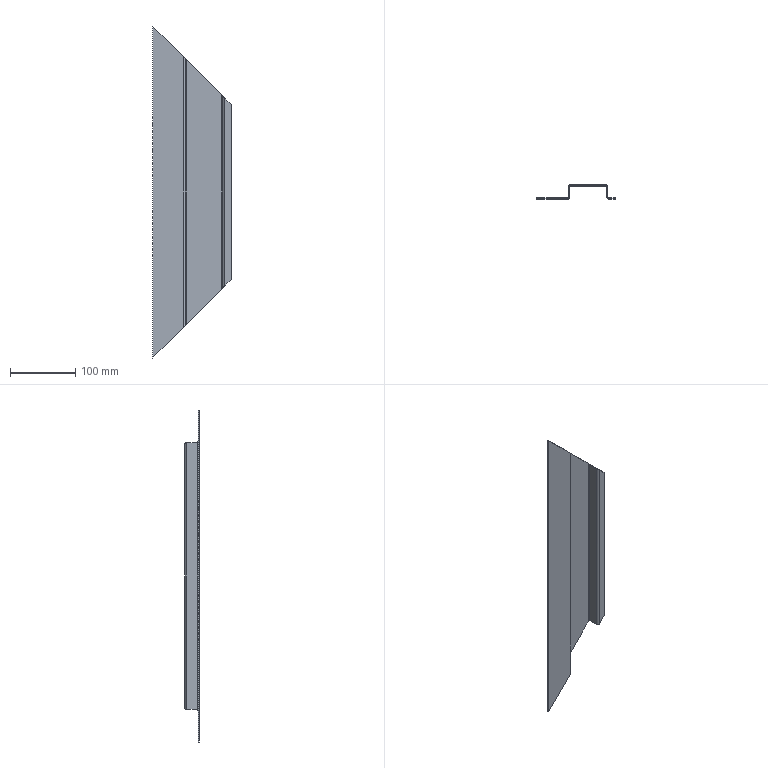Part | STEP file | 750038523 | 1 solid | 38 faces | box 120 x 21.5 x 508 mm | volume 88776 mm3 | plane 22 | cylinder 8 | spline 8 | commonest cylinder face diameters 3 x4 6 x4
STEP:
#1=CARTESIAN_POINT('',(-120.,-1.5,254.));
#2=VERTEX_POINT('',#1);
#3=CARTESIAN_POINT('',(-120.,-1.5,-254.));
#4=VERTEX_POINT('',#3);
#5=CARTESIAN_POINT('',(-120.,-1.5,254.));
#6=DIRECTION('',(0.,0.,-1.));
#7=VECTOR('',#6,1000.);
#8=LINE('',#5,#7);
#9=EDGE_CURVE('',#2,#4,#8,.T.);
#10=ORIENTED_EDGE('',*,*,#9,.T.);
#11=CARTESIAN_POINT('',(-73.,-1.5,-207.));
#12=VERTEX_POINT('',#11);
#13=CARTESIAN_POINT('',(-120.,-1.5,-254.));
#14=DIRECTION('',(0.7071,0.,0.7071));
#15=VECTOR('',#14,1000.);
#16=LINE('',#13,#15);
#17=EDGE_CURVE('',#4,#12,#16,.T.);
#18=ORIENTED_EDGE('',*,*,#17,.T.);
#19=CARTESIAN_POINT('',(-73.,-1.5,207.));
#20=VERTEX_POINT('',#19);
#21=CARTESIAN_POINT('',(-73.,-1.5,254.));
#22=DIRECTION('',(0.,0.,1.));
#23=VECTOR('',#22,1000.);
#24=LINE('',#21,#23);
#25=EDGE_CURVE('',#12,#20,#24,.T.);
#26=ORIENTED_EDGE('',*,*,#25,.T.);
#27=CARTESIAN_POINT('',(-73.,-1.5,207.));
#28=DIRECTION('',(-0.7071,0.,0.7071));
#29=VECTOR('',#28,1000.);
#30=LINE('',#27,#29);
#31=EDGE_CURVE('',#20,#2,#30,.T.);
#32=ORIENTED_EDGE('',*,*,#31,.T.);
#33=EDGE_LOOP('',(#10,#18,#26,#32));
#34=FACE_OUTER_BOUND('',#33,.T.);
#35=CARTESIAN_POINT('',(-71.5,-1.5,254.));
#36=DIRECTION('',(0.,-1.,0.));
#37=DIRECTION('',(1.,0.,0.));
#38=AXIS2_PLACEMENT_3D('',#35,#36,#37);
#39=PLANE('',#38);
#40=ADVANCED_FACE('',(#34),#39,.T.);
#41=CARTESIAN_POINT('',(-73.,0.,-207.));
#42=VERTEX_POINT('',#41);
#43=CARTESIAN_POINT('',(-73.,-0.75,-207.));
#44=DIRECTION('',(0.,-1.,0.));
#45=VECTOR('',#44,1000.);
#46=LINE('',#43,#45);
#47=EDGE_CURVE('',#42,#12,#46,.T.);
#48=ORIENTED_EDGE('',*,*,#47,.T.);
#49=ORIENTED_EDGE('',*,*,#17,.F.);
#50=CARTESIAN_POINT('',(-120.,0.,-254.));
#51=VERTEX_POINT('',#50);
#52=CARTESIAN_POINT('',(-120.,0.,-254.));
#53=DIRECTION('',(0.,1.,0.));
#54=VECTOR('',#53,1000.);
#55=LINE('',#52,#54);
#56=EDGE_CURVE('',#4,#51,#55,.T.);
#57=ORIENTED_EDGE('',*,*,#56,.T.);
#58=CARTESIAN_POINT('',(158.25,0.,24.25));
#59=DIRECTION('',(0.7071,0.,0.7071));
#60=VECTOR('',#59,1000.);
#61=LINE('',#58,#60);
#62=EDGE_CURVE('',#51,#42,#61,.T.);
#63=ORIENTED_EDGE('',*,*,#62,.T.);
#64=EDGE_LOOP('',(#48,#49,#57,#63));
#65=FACE_OUTER_BOUND('',#64,.T.);
#66=CARTESIAN_POINT('',(158.25,0.,24.25));
#67=DIRECTION('',(0.7071,0.,-0.7071));
#68=DIRECTION('',(-0.7071,0.,-0.7071));
#69=AXIS2_PLACEMENT_3D('',#66,#67,#68);
#70=PLANE('',#69);
#71=ADVANCED_FACE('',(#65),#70,.T.);
#72=ORIENTED_EDGE('',*,*,#56,.F.);
#73=ORIENTED_EDGE('',*,*,#9,.F.);
#74=CARTESIAN_POINT('',(-120.,0.,254.));
#75=VERTEX_POINT('',#74);
#76=CARTESIAN_POINT('',(-120.,0.,254.));
#77=DIRECTION('',(0.,1.,0.));
#78=VECTOR('',#77,1000.);
#79=LINE('',#76,#78);
#80=EDGE_CURVE('',#2,#75,#79,.T.);
#81=ORIENTED_EDGE('',*,*,#80,.T.);
#82=CARTESIAN_POINT('',(-120.,0.,254.));
#83=DIRECTION('',(0.,0.,-1.));
#84=VECTOR('',#83,1000.);
#85=LINE('',#82,#84);
#86=EDGE_CURVE('',#75,#51,#85,.T.);
#87=ORIENTED_EDGE('',*,*,#86,.T.);
#88=EDGE_LOOP('',(#72,#73,#81,#87));
#89=FACE_OUTER_BOUND('',#88,.T.);
#90=CARTESIAN_POINT('',(-120.,0.,254.));
#91=DIRECTION('',(-1.,0.,0.));
#92=DIRECTION('',(0.,-1.,0.));
#93=AXIS2_PLACEMENT_3D('',#90,#91,#92);
#94=PLANE('',#93);
#95=ADVANCED_FACE('',(#89),#94,.T.);
#96=ORIENTED_EDGE('',*,*,#80,.F.);
#97=ORIENTED_EDGE('',*,*,#31,.F.);
#98=CARTESIAN_POINT('',(-73.,0.,207.));
#99=VERTEX_POINT('',#98);
#100=CARTESIAN_POINT('',(-73.,-0.75,207.));
#101=DIRECTION('',(0.,1.,0.));
#102=VECTOR('',#101,1000.);
#103=LINE('',#100,#102);
#104=EDGE_CURVE('',#20,#99,#103,.T.);
#105=ORIENTED_EDGE('',*,*,#104,.T.);
#106=CARTESIAN_POINT('',(-95.75,0.,229.75));
#107=DIRECTION('',(-0.7071,0.,0.7071));
#108=VECTOR('',#107,1000.);
#109=LINE('',#106,#108);
#110=EDGE_CURVE('',#99,#75,#109,.T.);
#111=ORIENTED_EDGE('',*,*,#110,.T.);
#112=EDGE_LOOP('',(#96,#97,#105,#111));
#113=FACE_OUTER_BOUND('',#112,.T.);
#114=CARTESIAN_POINT('',(-95.75,0.,229.75));
#115=DIRECTION('',(0.7071,0.,0.7071));
#116=DIRECTION('',(0.7071,0.,-0.7071));
#117=AXIS2_PLACEMENT_3D('',#114,#115,#116);
#118=PLANE('',#117);
#119=ADVANCED_FACE('',(#113),#118,.T.);
#120=ORIENTED_EDGE('',*,*,#25,.F.);
#121=CARTESIAN_POINT('',(-70.,1.5,-204.));
#122=VERTEX_POINT('',#121);
#123=CARTESIAN_POINT('',(-73.,-1.5,-207.));
#124=CARTESIAN_POINT('',(-71.,-1.5,-205.));
#125=CARTESIAN_POINT('',(-70.,0.,-204.));
#126=CARTESIAN_POINT('',(-70.,1.5,-204.));
#127=(BOUNDED_CURVE()B_SPLINE_CURVE(3,(#123,#124,#125,#126),.UNSPECIFIED.,.F.,.T.)B_SPLINE_CURVE_WITH_KNOTS((4,4),(0.,0.005675),.UNSPECIFIED.)CURVE()GEOMETRIC_REPRESENTATION_ITEM()RATIONAL_B_SPLINE_CURVE((0.5,0.5,0.6667,1.))REPRESENTATION_ITEM(''));
#128=EDGE_CURVE('',#12,#122,#127,.T.);
#129=ORIENTED_EDGE('',*,*,#128,.T.);
#130=CARTESIAN_POINT('',(-70.,1.5,204.));
#131=VERTEX_POINT('',#130);
#132=CARTESIAN_POINT('',(-70.,1.5,254.));
#133=DIRECTION('',(0.,0.,1.));
#134=VECTOR('',#133,1000.);
#135=LINE('',#132,#134);
#136=EDGE_CURVE('',#122,#131,#135,.T.);
#137=ORIENTED_EDGE('',*,*,#136,.T.);
#138=CARTESIAN_POINT('',(-70.,1.5,204.));
#139=CARTESIAN_POINT('',(-70.,0.,204.));
#140=CARTESIAN_POINT('',(-71.,-1.5,205.));
#141=CARTESIAN_POINT('',(-73.,-1.5,207.));
#142=(BOUNDED_CURVE()B_SPLINE_CURVE(3,(#138,#139,#140,#141),.UNSPECIFIED.,.F.,.T.)B_SPLINE_CURVE_WITH_KNOTS((4,4),(0.,0.005725),.UNSPECIFIED.)CURVE()GEOMETRIC_REPRESENTATION_ITEM()RATIONAL_B_SPLINE_CURVE((1.,0.6667,0.5,0.5))REPRESENTATION_ITEM(''));
#143=EDGE_CURVE('',#131,#20,#142,.T.);
#144=ORIENTED_EDGE('',*,*,#143,.T.);
#145=EDGE_LOOP('',(#120,#129,#137,#144));
#146=FACE_OUTER_BOUND('',#145,.T.);
#147=CARTESIAN_POINT('',(-73.,1.5,254.));
#148=DIRECTION('',(0.,0.,-1.));
#149=DIRECTION('',(-1.,0.,0.));
#150=AXIS2_PLACEMENT_3D('',#147,#148,#149);
#151=CYLINDRICAL_SURFACE('',#150,3.);
#152=ADVANCED_FACE('',(#146),#151,.T.);
#153=CARTESIAN_POINT('',(-73.,0.,254.));
#154=DIRECTION('',(0.,0.,1.));
#155=VECTOR('',#154,1000.);
#156=LINE('',#153,#155);
#157=EDGE_CURVE('',#42,#99,#156,.T.);
#158=ORIENTED_EDGE('',*,*,#157,.F.);
#159=ORIENTED_EDGE('',*,*,#62,.F.);
#160=ORIENTED_EDGE('',*,*,#86,.F.);
#161=ORIENTED_EDGE('',*,*,#110,.F.);
#162=EDGE_LOOP('',(#158,#159,#160,#161));
#163=FACE_OUTER_BOUND('',#162,.T.);
#164=CARTESIAN_POINT('',(-71.5,0.,254.));
#165=DIRECTION('',(0.,-1.,0.));
#166=DIRECTION('',(1.,0.,0.));
#167=AXIS2_PLACEMENT_3D('',#164,#165,#166);
#168=PLANE('',#167);
#169=ADVANCED_FACE('',(#163),#168,.F.);
#170=ORIENTED_EDGE('',*,*,#128,.F.);
#171=ORIENTED_EDGE('',*,*,#47,.F.);
#172=CARTESIAN_POINT('',(-71.5,1.5,-204.));
#173=VERTEX_POINT('',#172);
#174=CARTESIAN_POINT('',(-71.5,1.5,-204.));
#175=CARTESIAN_POINT('',(-71.5,0.75,-204.));
#176=CARTESIAN_POINT('',(-72.,0.,-205.));
#177=CARTESIAN_POINT('',(-73.,0.,-207.));
#178=(BOUNDED_CURVE()B_SPLINE_CURVE(3,(#174,#175,#176,#177),.UNSPECIFIED.,.F.,.F.)B_SPLINE_CURVE_WITH_KNOTS((4,4),(0.,0.003968),.UNSPECIFIED.)CURVE()GEOMETRIC_REPRESENTATION_ITEM()RATIONAL_B_SPLINE_CURVE((1.,0.6667,0.5,0.5))REPRESENTATION_ITEM(''));
#179=EDGE_CURVE('',#173,#42,#178,.T.);
#180=ORIENTED_EDGE('',*,*,#179,.F.);
#181=CARTESIAN_POINT('',(-70.,1.5,-204.));
#182=DIRECTION('',(-1.,0.,0.));
#183=VECTOR('',#182,1000.);
#184=LINE('',#181,#183);
#185=EDGE_CURVE('',#122,#173,#184,.T.);
#186=ORIENTED_EDGE('',*,*,#185,.F.);
#187=EDGE_LOOP('',(#170,#171,#180,#186));
#188=FACE_OUTER_BOUND('',#187,.T.);
#189=CARTESIAN_POINT('',(-76.,1.5,-210.));
#190=CARTESIAN_POINT('',(-75.5,1.5,-210.));
#191=CARTESIAN_POINT('',(-75.,1.5,-210.));
#192=CARTESIAN_POINT('',(-74.5,1.5,-210.));
#193=CARTESIAN_POINT('',(-76.,-4.5,-210.));
#194=CARTESIAN_POINT('',(-75.5,-3.5,-210.));
#195=CARTESIAN_POINT('',(-75.,-2.5,-210.));
#196=CARTESIAN_POINT('',(-74.5,-1.5,-210.));
#197=CARTESIAN_POINT('',(-70.,-4.5,-204.));
#198=CARTESIAN_POINT('',(-70.5,-3.5,-204.));
#199=CARTESIAN_POINT('',(-71.,-2.5,-204.));
#200=CARTESIAN_POINT('',(-71.5,-1.5,-204.));
#201=CARTESIAN_POINT('',(-70.,1.5,-204.));
#202=CARTESIAN_POINT('',(-70.5,1.5,-204.));
#203=CARTESIAN_POINT('',(-71.,1.5,-204.));
#204=CARTESIAN_POINT('',(-71.5,1.5,-204.));
#205=CARTESIAN_POINT('',(-70.,7.5,-204.));
#206=CARTESIAN_POINT('',(-70.5,6.5,-204.));
#207=CARTESIAN_POINT('',(-71.,5.5,-204.));
#208=CARTESIAN_POINT('',(-71.5,4.5,-204.));
#209=CARTESIAN_POINT('',(-76.,7.5,-210.));
#210=CARTESIAN_POINT('',(-75.5,6.5,-210.));
#211=CARTESIAN_POINT('',(-75.,5.5,-210.));
#212=CARTESIAN_POINT('',(-74.5,4.5,-210.));
#213=CARTESIAN_POINT('',(-76.,1.5,-210.));
#214=CARTESIAN_POINT('',(-75.5,1.5,-210.));
#215=CARTESIAN_POINT('',(-75.,1.5,-210.));
#216=CARTESIAN_POINT('',(-74.5,1.5,-210.));
#217=(BOUNDED_SURFACE()B_SPLINE_SURFACE(3,3,((#189,#190,#191,#192),(#193,#194,#195,#196),(#197,#198,#199,#200),(#201,#202,#203,#204),(#205,#206,#207,#208),(#209,#210,#211,#212),(#213,#214,#215,#216)),.UNSPECIFIED.,.T.,.F.,.F.)B_SPLINE_SURFACE_WITH_KNOTS((4,3,4),(4,4),(0.,0.5,1.),(0.,1.),.UNSPECIFIED.)GEOMETRIC_REPRESENTATION_ITEM()RATIONAL_B_SPLINE_SURFACE(((1.,1.,1.,1.),(0.3333,0.3333,0.3333,0.3333),(0.3333,0.3333,0.3333,0.3333),(1.,1.,1.,1.),(0.3333,0.3333,0.3333,0.3333),(0.3333,0.3333,0.3333,0.3333),(1.,1.,1.,1.)))REPRESENTATION_ITEM('')SURFACE());
#218=ADVANCED_FACE('',(#188),#217,.F.);
#219=ORIENTED_EDGE('',*,*,#104,.F.);
#220=ORIENTED_EDGE('',*,*,#143,.F.);
#221=CARTESIAN_POINT('',(-71.5,1.5,204.));
#222=VERTEX_POINT('',#221);
#223=CARTESIAN_POINT('',(-70.,1.5,204.));
#224=DIRECTION('',(1.,0.,0.));
#225=VECTOR('',#224,1000.);
#226=LINE('',#223,#225);
#227=EDGE_CURVE('',#222,#131,#226,.T.);
#228=ORIENTED_EDGE('',*,*,#227,.F.);
#229=CARTESIAN_POINT('',(-73.,0.,207.));
#230=CARTESIAN_POINT('',(-72.,0.,205.));
#231=CARTESIAN_POINT('',(-71.5,0.75,204.));
#232=CARTESIAN_POINT('',(-71.5,1.5,204.));
#233=(BOUNDED_CURVE()B_SPLINE_CURVE(3,(#229,#230,#231,#232),.UNSPECIFIED.,.F.,.F.)B_SPLINE_CURVE_WITH_KNOTS((4,4),(0.,0.003921),.UNSPECIFIED.)CURVE()GEOMETRIC_REPRESENTATION_ITEM()RATIONAL_B_SPLINE_CURVE((0.5,0.5,0.6667,1.))REPRESENTATION_ITEM(''));
#234=EDGE_CURVE('',#99,#222,#233,.T.);
#235=ORIENTED_EDGE('',*,*,#234,.F.);
#236=EDGE_LOOP('',(#219,#220,#228,#235));
#237=FACE_OUTER_BOUND('',#236,.T.);
#238=CARTESIAN_POINT('',(-70.,1.5,204.));
#239=CARTESIAN_POINT('',(-70.5,1.5,204.));
#240=CARTESIAN_POINT('',(-71.,1.5,204.));
#241=CARTESIAN_POINT('',(-71.5,1.5,204.));
#242=CARTESIAN_POINT('',(-70.,-4.5,204.));
#243=CARTESIAN_POINT('',(-70.5,-3.5,204.));
#244=CARTESIAN_POINT('',(-71.,-2.5,204.));
#245=CARTESIAN_POINT('',(-71.5,-1.5,204.));
#246=CARTESIAN_POINT('',(-76.,-4.5,210.));
#247=CARTESIAN_POINT('',(-75.5,-3.5,210.));
#248=CARTESIAN_POINT('',(-75.,-2.5,210.));
#249=CARTESIAN_POINT('',(-74.5,-1.5,210.));
#250=CARTESIAN_POINT('',(-76.,1.5,210.));
#251=CARTESIAN_POINT('',(-75.5,1.5,210.));
#252=CARTESIAN_POINT('',(-75.,1.5,210.));
#253=CARTESIAN_POINT('',(-74.5,1.5,210.));
#254=CARTESIAN_POINT('',(-76.,7.5,210.));
#255=CARTESIAN_POINT('',(-75.5,6.5,210.));
#256=CARTESIAN_POINT('',(-75.,5.5,210.));
#257=CARTESIAN_POINT('',(-74.5,4.5,210.));
#258=CARTESIAN_POINT('',(-70.,7.5,204.));
#259=CARTESIAN_POINT('',(-70.5,6.5,204.));
#260=CARTESIAN_POINT('',(-71.,5.5,204.));
#261=CARTESIAN_POINT('',(-71.5,4.5,204.));
#262=CARTESIAN_POINT('',(-70.,1.5,204.));
#263=CARTESIAN_POINT('',(-70.5,1.5,204.));
#264=CARTESIAN_POINT('',(-71.,1.5,204.));
#265=CARTESIAN_POINT('',(-71.5,1.5,204.));
#266=(BOUNDED_SURFACE()B_SPLINE_SURFACE(3,3,((#238,#239,#240,#241),(#242,#243,#244,#245),(#246,#247,#248,#249),(#250,#251,#252,#253),(#254,#255,#256,#257),(#258,#259,#260,#261),(#262,#263,#264,#265)),.UNSPECIFIED.,.T.,.F.,.F.)B_SPLINE_SURFACE_WITH_KNOTS((4,3,4),(4,4),(0.,0.5,1.),(0.,1.),.UNSPECIFIED.)GEOMETRIC_REPRESENTATION_ITEM()RATIONAL_B_SPLINE_SURFACE(((1.,1.,1.,1.),(0.3333,0.3333,0.3333,0.3333),(0.3333,0.3333,0.3333,0.3333),(1.,1.,1.,1.),(0.3333,0.3333,0.3333,0.3333),(0.3333,0.3333,0.3333,0.3333),(1.,1.,1.,1.)))REPRESENTATION_ITEM('')SURFACE());
#267=ADVANCED_FACE('',(#237),#266,.F.);
#268=ORIENTED_EDGE('',*,*,#136,.F.);
#269=CARTESIAN_POINT('',(-70.,17.,-204.));
#270=VERTEX_POINT('',#269);
#271=CARTESIAN_POINT('',(-70.,20.,-204.));
#272=DIRECTION('',(0.,1.,0.));
#273=VECTOR('',#272,1000.);
#274=LINE('',#271,#273);
#275=EDGE_CURVE('',#122,#270,#274,.T.);
#276=ORIENTED_EDGE('',*,*,#275,.T.);
#277=CARTESIAN_POINT('',(-70.,17.,204.));
#278=VERTEX_POINT('',#277);
#279=CARTESIAN_POINT('',(-70.,17.,254.));
#280=DIRECTION('',(0.,0.,1.));
#281=VECTOR('',#280,1000.);
#282=LINE('',#279,#281);
#283=EDGE_CURVE('',#270,#278,#282,.T.);
#284=ORIENTED_EDGE('',*,*,#283,.T.);
#285=CARTESIAN_POINT('',(-70.,20.,204.));
#286=DIRECTION('',(0.,-1.,0.));
#287=VECTOR('',#286,1000.);
#288=LINE('',#285,#287);
#289=EDGE_CURVE('',#278,#131,#288,.T.);
#290=ORIENTED_EDGE('',*,*,#289,.T.);
#291=EDGE_LOOP('',(#268,#276,#284,#290));
#292=FACE_OUTER_BOUND('',#291,.T.);
#293=CARTESIAN_POINT('',(-70.,20.,254.));
#294=DIRECTION('',(1.,0.,0.));
#295=DIRECTION('',(0.,0.,-1.));
#296=AXIS2_PLACEMENT_3D('',#293,#294,#295);
#297=PLANE('',#296);
#298=ADVANCED_FACE('',(#292),#297,.T.);
#299=CARTESIAN_POINT('',(-71.5,1.5,254.));
#300=DIRECTION('',(0.,0.,1.));
#301=VECTOR('',#300,1000.);
#302=LINE('',#299,#301);
#303=EDGE_CURVE('',#173,#222,#302,.T.);
#304=ORIENTED_EDGE('',*,*,#303,.F.);
#305=ORIENTED_EDGE('',*,*,#179,.T.);
#306=ORIENTED_EDGE('',*,*,#157,.T.);
#307=ORIENTED_EDGE('',*,*,#234,.T.);
#308=EDGE_LOOP('',(#304,#305,#306,#307));
#309=FACE_OUTER_BOUND('',#308,.T.);
#310=CARTESIAN_POINT('',(-73.,1.5,254.));
#311=DIRECTION('',(0.,0.,-1.));
#312=DIRECTION('',(-1.,0.,0.));
#313=AXIS2_PLACEMENT_3D('',#310,#311,#312);
#314=CYLINDRICAL_SURFACE('',#313,1.5);
#315=ADVANCED_FACE('',(#309),#314,.F.);
#316=ORIENTED_EDGE('',*,*,#185,.T.);
#317=CARTESIAN_POINT('',(-71.5,17.,-204.));
#318=VERTEX_POINT('',#317);
#319=CARTESIAN_POINT('',(-71.5,20.,-204.));
#320=DIRECTION('',(0.,1.,0.));
#321=VECTOR('',#320,1000.);
#322=LINE('',#319,#321);
#323=EDGE_CURVE('',#173,#318,#322,.T.);
#324=ORIENTED_EDGE('',*,*,#323,.T.);
#325=CARTESIAN_POINT('',(-70.75,17.,-204.));
#326=DIRECTION('',(1.,0.,0.));
#327=VECTOR('',#326,1000.);
#328=LINE('',#325,#327);
#329=EDGE_CURVE('',#318,#270,#328,.T.);
#330=ORIENTED_EDGE('',*,*,#329,.T.);
#331=ORIENTED_EDGE('',*,*,#275,.F.);
#332=EDGE_LOOP('',(#316,#324,#330,#331));
#333=FACE_OUTER_BOUND('',#332,.T.);
#334=CARTESIAN_POINT('',(-70.,20.,-204.));
#335=DIRECTION('',(0.,0.,-1.));
#336=DIRECTION('',(-1.,0.,0.));
#337=AXIS2_PLACEMENT_3D('',#334,#335,#336);
#338=PLANE('',#337);
#339=ADVANCED_FACE('',(#333),#338,.T.);
#340=CARTESIAN_POINT('',(-71.5,17.,204.));
#341=VERTEX_POINT('',#340);
#342=CARTESIAN_POINT('',(-70.75,17.,204.));
#343=DIRECTION('',(-1.,0.,0.));
#344=VECTOR('',#343,1000.);
#345=LINE('',#342,#344);
#346=EDGE_CURVE('',#278,#341,#345,.T.);
#347=ORIENTED_EDGE('',*,*,#346,.T.);
#348=CARTESIAN_POINT('',(-71.5,20.,204.));
#349=DIRECTION('',(0.,-1.,0.));
#350=VECTOR('',#349,1000.);
#351=LINE('',#348,#350);
#352=EDGE_CURVE('',#341,#222,#351,.T.);
#353=ORIENTED_EDGE('',*,*,#352,.T.);
#354=ORIENTED_EDGE('',*,*,#227,.T.);
#355=ORIENTED_EDGE('',*,*,#289,.F.);
#356=EDGE_LOOP('',(#347,#353,#354,#355));
#357=FACE_OUTER_BOUND('',#356,.T.);
#358=CARTESIAN_POINT('',(-70.,20.,204.));
#359=DIRECTION('',(0.,0.,1.));
#360=DIRECTION('',(1.,0.,0.));
#361=AXIS2_PLACEMENT_3D('',#358,#359,#360);
#362=PLANE('',#361);
#363=ADVANCED_FACE('',(#357),#362,.T.);
#364=CARTESIAN_POINT('',(-68.5,18.5,202.5));
#365=VERTEX_POINT('',#364);
#366=CARTESIAN_POINT('',(-70.,17.,204.));
#367=CARTESIAN_POINT('',(-70.,17.75,204.));
#368=CARTESIAN_POINT('',(-69.5,18.5,203.5));
#369=CARTESIAN_POINT('',(-68.5,18.5,202.5));
#370=(BOUNDED_CURVE()B_SPLINE_CURVE(3,(#366,#367,#368,#369),.UNSPECIFIED.,.F.,.F.)B_SPLINE_CURVE_WITH_KNOTS((4,4),(0.,0.002854),.UNSPECIFIED.)CURVE()GEOMETRIC_REPRESENTATION_ITEM()RATIONAL_B_SPLINE_CURVE((1.,0.6667,0.5,0.5))REPRESENTATION_ITEM(''));
#371=EDGE_CURVE('',#278,#365,#370,.T.);
#372=ORIENTED_EDGE('',*,*,#371,.F.);
#373=ORIENTED_EDGE('',*,*,#283,.F.);
#374=CARTESIAN_POINT('',(-68.5,18.5,-202.5));
#375=VERTEX_POINT('',#374);
#376=CARTESIAN_POINT('',(-68.5,18.5,-202.5));
#377=CARTESIAN_POINT('',(-69.5,18.5,-203.5));
#378=CARTESIAN_POINT('',(-70.,17.75,-204.));
#379=CARTESIAN_POINT('',(-70.,17.,-204.));
#380=(BOUNDED_CURVE()B_SPLINE_CURVE(3,(#376,#377,#378,#379),.UNSPECIFIED.,.F.,.F.)B_SPLINE_CURVE_WITH_KNOTS((4,4),(0.,0.002839),.UNSPECIFIED.)CURVE()GEOMETRIC_REPRESENTATION_ITEM()RATIONAL_B_SPLINE_CURVE((0.5,0.5,0.6667,1.))REPRESENTATION_ITEM(''));
#381=EDGE_CURVE('',#375,#270,#380,.T.);
#382=ORIENTED_EDGE('',*,*,#381,.F.);
#383=CARTESIAN_POINT('',(-68.5,18.5,254.));
#384=DIRECTION('',(0.,0.,-1.));
#385=VECTOR('',#384,1000.);
#386=LINE('',#383,#385);
#387=EDGE_CURVE('',#365,#375,#386,.T.);
#388=ORIENTED_EDGE('',*,*,#387,.F.);
#389=EDGE_LOOP('',(#372,#373,#382,#388));
#390=FACE_OUTER_BOUND('',#389,.T.);
#391=CARTESIAN_POINT('',(-68.5,17.,254.));
#392=DIRECTION('',(0.,0.,-1.));
#393=DIRECTION('',(-1.,0.,0.));
#394=AXIS2_PLACEMENT_3D('',#391,#392,#393);
#395=CYLINDRICAL_SURFACE('',#394,1.5);
#396=ADVANCED_FACE('',(#390),#395,.F.);
#397=CARTESIAN_POINT('',(-71.5,17.,254.));
#398=DIRECTION('',(0.,0.,1.));
#399=VECTOR('',#398,1000.);
#400=LINE('',#397,#399);
#401=EDGE_CURVE('',#318,#341,#400,.T.);
#402=ORIENTED_EDGE('',*,*,#401,.F.);
#403=ORIENTED_EDGE('',*,*,#323,.F.);
#404=ORIENTED_EDGE('',*,*,#303,.T.);
#405=ORIENTED_EDGE('',*,*,#352,.F.);
#406=EDGE_LOOP('',(#402,#403,#404,#405));
#407=FACE_OUTER_BOUND('',#406,.T.);
#408=CARTESIAN_POINT('',(-71.5,20.,254.));
#409=DIRECTION('',(1.,0.,0.));
#410=DIRECTION('',(0.,0.,-1.));
#411=AXIS2_PLACEMENT_3D('',#408,#409,#410);
#412=PLANE('',#411);
#413=ADVANCED_FACE('',(#407),#412,.F.);
#414=ORIENTED_EDGE('',*,*,#387,.T.);
#415=CARTESIAN_POINT('',(-14.5,18.5,-148.5));
#416=VERTEX_POINT('',#415);
#417=CARTESIAN_POINT('',(-68.5,18.5,-202.5));
#418=DIRECTION('',(0.7071,0.,0.7071));
#419=VECTOR('',#418,1000.);
#420=LINE('',#417,#419);
#421=EDGE_CURVE('',#375,#416,#420,.T.);
#422=ORIENTED_EDGE('',*,*,#421,.T.);
#423=CARTESIAN_POINT('',(-14.5,18.5,148.5));
#424=VERTEX_POINT('',#423);
#425=CARTESIAN_POINT('',(-14.5,18.5,254.));
#426=DIRECTION('',(0.,0.,1.));
#427=VECTOR('',#426,1000.);
#428=LINE('',#425,#427);
#429=EDGE_CURVE('',#416,#424,#428,.T.);
#430=ORIENTED_EDGE('',*,*,#429,.T.);
#431=CARTESIAN_POINT('',(-14.5,18.5,148.5));
#432=DIRECTION('',(-0.7071,0.,0.7071));
#433=VECTOR('',#432,1000.);
#434=LINE('',#431,#433);
#435=EDGE_CURVE('',#424,#365,#434,.T.);
#436=ORIENTED_EDGE('',*,*,#435,.T.);
#437=EDGE_LOOP('',(#414,#422,#430,#436));
#438=FACE_OUTER_BOUND('',#437,.T.);
#439=CARTESIAN_POINT('',(-11.5,18.5,254.));
#440=DIRECTION('',(0.,-1.,0.));
#441=DIRECTION('',(1.,0.,0.));
#442=AXIS2_PLACEMENT_3D('',#439,#440,#441);
#443=PLANE('',#442);
#444=ADVANCED_FACE('',(#438),#443,.T.);
#445=ORIENTED_EDGE('',*,*,#371,.T.);
#446=CARTESIAN_POINT('',(-68.5,20.,202.5));
#447=VERTEX_POINT('',#446);
#448=CARTESIAN_POINT('',(-68.5,19.25,202.5));
#449=DIRECTION('',(0.,-1.,0.));
#450=VECTOR('',#449,1000.);
#451=LINE('',#448,#450);
#452=EDGE_CURVE('',#447,#365,#451,.T.);
#453=ORIENTED_EDGE('',*,*,#452,.F.);
#454=CARTESIAN_POINT('',(-71.5,17.,204.));
#455=CARTESIAN_POINT('',(-71.5,18.5,204.));
#456=CARTESIAN_POINT('',(-70.5,20.,203.5));
#457=CARTESIAN_POINT('',(-68.5,20.,202.5));
#458=(BOUNDED_CURVE()B_SPLINE_CURVE(3,(#454,#455,#456,#457),.UNSPECIFIED.,.F.,.F.)B_SPLINE_CURVE_WITH_KNOTS((4,4),(0.,0.00499),.UNSPECIFIED.)CURVE()GEOMETRIC_REPRESENTATION_ITEM()RATIONAL_B_SPLINE_CURVE((1.,0.6667,0.5,0.5))REPRESENTATION_ITEM(''));
#459=EDGE_CURVE('',#341,#447,#458,.T.);
#460=ORIENTED_EDGE('',*,*,#459,.F.);
#461=ORIENTED_EDGE('',*,*,#346,.F.);
#462=EDGE_LOOP('',(#445,#453,#460,#461));
#463=FACE_OUTER_BOUND('',#462,.T.);
#464=CARTESIAN_POINT('',(-67.,17.,201.));
#465=CARTESIAN_POINT('',(-66.5,17.,201.));
#466=CARTESIAN_POINT('',(-66.,17.,201.));
#467=CARTESIAN_POINT('',(-65.5,17.,201.));
#468=CARTESIAN_POINT('',(-67.,20.,201.));
#469=CARTESIAN_POINT('',(-66.5,21.,201.));
#470=CARTESIAN_POINT('',(-66.,22.,201.));
#471=CARTESIAN_POINT('',(-65.5,23.,201.));
#472=CARTESIAN_POINT('',(-70.,20.,204.));
#473=CARTESIAN_POINT('',(-70.5,21.,204.));
#474=CARTESIAN_POINT('',(-71.,22.,204.));
#475=CARTESIAN_POINT('',(-71.5,23.,204.));
#476=CARTESIAN_POINT('',(-70.,17.,204.));
#477=CARTESIAN_POINT('',(-70.5,17.,204.));
#478=CARTESIAN_POINT('',(-71.,17.,204.));
#479=CARTESIAN_POINT('',(-71.5,17.,204.));
#480=CARTESIAN_POINT('',(-70.,14.,204.));
#481=CARTESIAN_POINT('',(-70.5,13.,204.));
#482=CARTESIAN_POINT('',(-71.,12.,204.));
#483=CARTESIAN_POINT('',(-71.5,11.,204.));
#484=CARTESIAN_POINT('',(-67.,14.,201.));
#485=CARTESIAN_POINT('',(-66.5,13.,201.));
#486=CARTESIAN_POINT('',(-66.,12.,201.));
#487=CARTESIAN_POINT('',(-65.5,11.,201.));
#488=CARTESIAN_POINT('',(-67.,17.,201.));
#489=CARTESIAN_POINT('',(-66.5,17.,201.));
#490=CARTESIAN_POINT('',(-66.,17.,201.));
#491=CARTESIAN_POINT('',(-65.5,17.,201.));
#492=(BOUNDED_SURFACE()B_SPLINE_SURFACE(3,3,((#464,#465,#466,#467),(#468,#469,#470,#471),(#472,#473,#474,#475),(#476,#477,#478,#479),(#480,#481,#482,#483),(#484,#485,#486,#487),(#488,#489,#490,#491)),.UNSPECIFIED.,.T.,.F.,.T.)B_SPLINE_SURFACE_WITH_KNOTS((4,3,4),(4,4),(0.,0.5,1.),(0.,1.),.UNSPECIFIED.)GEOMETRIC_REPRESENTATION_ITEM()RATIONAL_B_SPLINE_SURFACE(((1.,1.,1.,1.),(0.3333,0.3333,0.3333,0.3333),(0.3333,0.3333,0.3333,0.3333),(1.,1.,1.,1.),(0.3333,0.3333,0.3333,0.3333),(0.3333,0.3333,0.3333,0.3333),(1.,1.,1.,1.)))REPRESENTATION_ITEM('')SURFACE());
#493=ADVANCED_FACE('',(#463),#492,.F.);
#494=ORIENTED_EDGE('',*,*,#381,.T.);
#495=ORIENTED_EDGE('',*,*,#329,.F.);
#496=CARTESIAN_POINT('',(-68.5,20.,-202.5));
#497=VERTEX_POINT('',#496);
#498=CARTESIAN_POINT('',(-68.5,20.,-202.5));
#499=CARTESIAN_POINT('',(-70.5,20.,-203.5));
#500=CARTESIAN_POINT('',(-71.5,18.5,-204.));
#501=CARTESIAN_POINT('',(-71.5,17.,-204.));
#502=(BOUNDED_CURVE()B_SPLINE_CURVE(3,(#498,#499,#500,#501),.UNSPECIFIED.,.F.,.F.)B_SPLINE_CURVE_WITH_KNOTS((4,4),(0.,0.004967),.UNSPECIFIED.)CURVE()GEOMETRIC_REPRESENTATION_ITEM()RATIONAL_B_SPLINE_CURVE((0.5,0.5,0.6667,1.))REPRESENTATION_ITEM(''));
#503=EDGE_CURVE('',#497,#318,#502,.T.);
#504=ORIENTED_EDGE('',*,*,#503,.F.);
#505=CARTESIAN_POINT('',(-68.5,19.25,-202.5));
#506=DIRECTION('',(0.,1.,0.));
#507=VECTOR('',#506,1000.);
#508=LINE('',#505,#507);
#509=EDGE_CURVE('',#375,#497,#508,.T.);
#510=ORIENTED_EDGE('',*,*,#509,.F.);
#511=EDGE_LOOP('',(#494,#495,#504,#510));
#512=FACE_OUTER_BOUND('',#511,.T.);
#513=CARTESIAN_POINT('',(-70.,17.,-204.));
#514=CARTESIAN_POINT('',(-70.5,17.,-204.));
#515=CARTESIAN_POINT('',(-71.,17.,-204.));
#516=CARTESIAN_POINT('',(-71.5,17.,-204.));
#517=CARTESIAN_POINT('',(-70.,20.,-204.));
#518=CARTESIAN_POINT('',(-70.5,21.,-204.));
#519=CARTESIAN_POINT('',(-71.,22.,-204.));
#520=CARTESIAN_POINT('',(-71.5,23.,-204.));
#521=CARTESIAN_POINT('',(-67.,20.,-201.));
#522=CARTESIAN_POINT('',(-66.5,21.,-201.));
#523=CARTESIAN_POINT('',(-66.,22.,-201.));
#524=CARTESIAN_POINT('',(-65.5,23.,-201.));
#525=CARTESIAN_POINT('',(-67.,17.,-201.));
#526=CARTESIAN_POINT('',(-66.5,17.,-201.));
#527=CARTESIAN_POINT('',(-66.,17.,-201.));
#528=CARTESIAN_POINT('',(-65.5,17.,-201.));
#529=CARTESIAN_POINT('',(-67.,14.,-201.));
#530=CARTESIAN_POINT('',(-66.5,13.,-201.));
#531=CARTESIAN_POINT('',(-66.,12.,-201.));
#532=CARTESIAN_POINT('',(-65.5,11.,-201.));
#533=CARTESIAN_POINT('',(-70.,14.,-204.));
#534=CARTESIAN_POINT('',(-70.5,13.,-204.));
#535=CARTESIAN_POINT('',(-71.,12.,-204.));
#536=CARTESIAN_POINT('',(-71.5,11.,-204.));
#537=CARTESIAN_POINT('',(-70.,17.,-204.));
#538=CARTESIAN_POINT('',(-70.5,17.,-204.));
#539=CARTESIAN_POINT('',(-71.,17.,-204.));
#540=CARTESIAN_POINT('',(-71.5,17.,-204.));
#541=(BOUNDED_SURFACE()B_SPLINE_SURFACE(3,3,((#513,#514,#515,#516),(#517,#518,#519,#520),(#521,#522,#523,#524),(#525,#526,#527,#528),(#529,#530,#531,#532),(#533,#534,#535,#536),(#537,#538,#539,#540)),.UNSPECIFIED.,.T.,.F.,.T.)B_SPLINE_SURFACE_WITH_KNOTS((4,3,4),(4,4),(0.,0.5,1.),(0.,1.),.UNSPECIFIED.)GEOMETRIC_REPRESENTATION_ITEM()RATIONAL_B_SPLINE_SURFACE(((1.,1.,1.,1.),(0.3333,0.3333,0.3333,0.3333),(0.3333,0.3333,0.3333,0.3333),(1.,1.,1.,1.),(0.3333,0.3333,0.3333,0.3333),(0.3333,0.3333,0.3333,0.3333),(1.,1.,1.,1.)))REPRESENTATION_ITEM('')SURFACE());
#542=ADVANCED_FACE('',(#512),#541,.F.);
#543=ORIENTED_EDGE('',*,*,#503,.T.);
#544=ORIENTED_EDGE('',*,*,#401,.T.);
#545=ORIENTED_EDGE('',*,*,#459,.T.);
#546=CARTESIAN_POINT('',(-68.5,20.,254.));
#547=DIRECTION('',(0.,0.,-1.));
#548=VECTOR('',#547,1000.);
#549=LINE('',#546,#548);
#550=EDGE_CURVE('',#447,#497,#549,.T.);
#551=ORIENTED_EDGE('',*,*,#550,.T.);
#552=EDGE_LOOP('',(#543,#544,#545,#551));
#553=FACE_OUTER_BOUND('',#552,.T.);
#554=CARTESIAN_POINT('',(-68.5,17.,254.));
#555=DIRECTION('',(0.,0.,-1.));
#556=DIRECTION('',(-1.,0.,0.));
#557=AXIS2_PLACEMENT_3D('',#554,#555,#556);
#558=CYLINDRICAL_SURFACE('',#557,3.);
#559=ADVANCED_FACE('',(#553),#558,.T.);
#560=CARTESIAN_POINT('',(-14.5,20.,-148.5));
#561=VERTEX_POINT('',#560);
#562=CARTESIAN_POINT('',(-14.5,19.25,-148.5));
#563=DIRECTION('',(0.,-1.,0.));
#564=VECTOR('',#563,1000.);
#565=LINE('',#562,#564);
#566=EDGE_CURVE('',#561,#416,#565,.T.);
#567=ORIENTED_EDGE('',*,*,#566,.T.);
#568=ORIENTED_EDGE('',*,*,#421,.F.);
#569=ORIENTED_EDGE('',*,*,#509,.T.);
#570=CARTESIAN_POINT('',(188.25,20.,54.25));
#571=DIRECTION('',(0.7071,0.,0.7071));
#572=VECTOR('',#571,1000.);
#573=LINE('',#570,#572);
#574=EDGE_CURVE('',#497,#561,#573,.T.);
#575=ORIENTED_EDGE('',*,*,#574,.T.);
#576=EDGE_LOOP('',(#567,#568,#569,#575));
#577=FACE_OUTER_BOUND('',#576,.T.);
#578=CARTESIAN_POINT('',(188.25,20.,54.25));
#579=DIRECTION('',(0.7071,0.,-0.7071));
#580=DIRECTION('',(-0.7071,0.,-0.7071));
#581=AXIS2_PLACEMENT_3D('',#578,#579,#580);
#582=PLANE('',#581);
#583=ADVANCED_FACE('',(#577),#582,.T.);
#584=ORIENTED_EDGE('',*,*,#452,.T.);
#585=ORIENTED_EDGE('',*,*,#435,.F.);
#586=CARTESIAN_POINT('',(-14.5,20.,148.5));
#587=VERTEX_POINT('',#586);
#588=CARTESIAN_POINT('',(-14.5,19.25,148.5));
#589=DIRECTION('',(0.,1.,0.));
#590=VECTOR('',#589,1000.);
#591=LINE('',#588,#590);
#592=EDGE_CURVE('',#424,#587,#591,.T.);
#593=ORIENTED_EDGE('',*,*,#592,.T.);
#594=CARTESIAN_POINT('',(-65.75,20.,199.75));
#595=DIRECTION('',(-0.7071,0.,0.7071));
#596=VECTOR('',#595,1000.);
#597=LINE('',#594,#596);
#598=EDGE_CURVE('',#587,#447,#597,.T.);
#599=ORIENTED_EDGE('',*,*,#598,.T.);
#600=EDGE_LOOP('',(#584,#585,#593,#599));
#601=FACE_OUTER_BOUND('',#600,.T.);
#602=CARTESIAN_POINT('',(-65.75,20.,199.75));
#603=DIRECTION('',(0.7071,0.,0.7071));
#604=DIRECTION('',(0.7071,0.,-0.7071));
#605=AXIS2_PLACEMENT_3D('',#602,#603,#604);
#606=PLANE('',#605);
#607=ADVANCED_FACE('',(#601),#606,.T.);
#608=CARTESIAN_POINT('',(-13.,17.,145.5));
#609=VERTEX_POINT('',#608);
#610=CARTESIAN_POINT('',(-14.5,18.5,148.5));
#611=CARTESIAN_POINT('',(-13.5,18.5,146.5));
#612=CARTESIAN_POINT('',(-13.,17.75,145.5));
#613=CARTESIAN_POINT('',(-13.,17.,145.5));
#614=(BOUNDED_CURVE()B_SPLINE_CURVE(3,(#610,#611,#612,#613),.UNSPECIFIED.,.F.,.F.)B_SPLINE_CURVE_WITH_KNOTS((4,4),(0.,0.003921),.UNSPECIFIED.)CURVE()GEOMETRIC_REPRESENTATION_ITEM()RATIONAL_B_SPLINE_CURVE((0.5,0.5,0.6667,1.))REPRESENTATION_ITEM(''));
#615=EDGE_CURVE('',#424,#609,#614,.T.);
#616=ORIENTED_EDGE('',*,*,#615,.F.);
#617=ORIENTED_EDGE('',*,*,#429,.F.);
#618=CARTESIAN_POINT('',(-13.,17.,-145.5));
#619=VERTEX_POINT('',#618);
#620=CARTESIAN_POINT('',(-13.,17.,-145.5));
#621=CARTESIAN_POINT('',(-13.,17.75,-145.5));
#622=CARTESIAN_POINT('',(-13.5,18.5,-146.5));
#623=CARTESIAN_POINT('',(-14.5,18.5,-148.5));
#624=(BOUNDED_CURVE()B_SPLINE_CURVE(3,(#620,#621,#622,#623),.UNSPECIFIED.,.F.,.F.)B_SPLINE_CURVE_WITH_KNOTS((4,4),(0.,0.003968),.UNSPECIFIED.)CURVE()GEOMETRIC_REPRESENTATION_ITEM()RATIONAL_B_SPLINE_CURVE((1.,0.6667,0.5,0.5))REPRESENTATION_ITEM(''));
#625=EDGE_CURVE('',#619,#416,#624,.T.);
#626=ORIENTED_EDGE('',*,*,#625,.F.);
#627=CARTESIAN_POINT('',(-13.,17.,254.));
#628=DIRECTION('',(0.,0.,-1.));
#629=VECTOR('',#628,1000.);
#630=LINE('',#627,#629);
#631=EDGE_CURVE('',#609,#619,#630,.T.);
#632=ORIENTED_EDGE('',*,*,#631,.F.);
#633=EDGE_LOOP('',(#616,#617,#626,#632));
#634=FACE_OUTER_BOUND('',#633,.T.);
#635=CARTESIAN_POINT('',(-14.5,17.,254.));
#636=DIRECTION('',(0.,0.,-1.));
#637=DIRECTION('',(-1.,0.,0.));
#638=AXIS2_PLACEMENT_3D('',#635,#636,#637);
#639=CYLINDRICAL_SURFACE('',#638,1.5);
#640=ADVANCED_FACE('',(#634),#639,.F.);
#641=CARTESIAN_POINT('',(-14.5,20.,254.));
#642=DIRECTION('',(0.,0.,1.));
#643=VECTOR('',#642,1000.);
#644=LINE('',#641,#643);
#645=EDGE_CURVE('',#561,#587,#644,.T.);
#646=ORIENTED_EDGE('',*,*,#645,.F.);
#647=ORIENTED_EDGE('',*,*,#574,.F.);
#648=ORIENTED_EDGE('',*,*,#550,.F.);
#649=ORIENTED_EDGE('',*,*,#598,.F.);
#650=EDGE_LOOP('',(#646,#647,#648,#649));
#651=FACE_OUTER_BOUND('',#650,.T.);
#652=CARTESIAN_POINT('',(-11.5,20.,254.));
#653=DIRECTION('',(0.,-1.,0.));
#654=DIRECTION('',(1.,0.,0.));
#655=AXIS2_PLACEMENT_3D('',#652,#653,#654);
#656=PLANE('',#655);
#657=ADVANCED_FACE('',(#651),#656,.F.);
#658=ORIENTED_EDGE('',*,*,#631,.T.);
#659=CARTESIAN_POINT('',(-13.,1.5,-145.5));
#660=VERTEX_POINT('',#659);
#661=CARTESIAN_POINT('',(-13.,0.,-145.5));
#662=DIRECTION('',(0.,-1.,0.));
#663=VECTOR('',#662,1000.);
#664=LINE('',#661,#663);
#665=EDGE_CURVE('',#619,#660,#664,.T.);
#666=ORIENTED_EDGE('',*,*,#665,.T.);
#667=CARTESIAN_POINT('',(-13.,1.5,145.5));
#668=VERTEX_POINT('',#667);
#669=CARTESIAN_POINT('',(-13.,1.5,254.));
#670=DIRECTION('',(0.,0.,1.));
#671=VECTOR('',#670,1000.);
#672=LINE('',#669,#671);
#673=EDGE_CURVE('',#660,#668,#672,.T.);
#674=ORIENTED_EDGE('',*,*,#673,.T.);
#675=CARTESIAN_POINT('',(-13.,0.,145.5));
#676=DIRECTION('',(0.,1.,0.));
#677=VECTOR('',#676,1000.);
#678=LINE('',#675,#677);
#679=EDGE_CURVE('',#668,#609,#678,.T.);
#680=ORIENTED_EDGE('',*,*,#679,.T.);
#681=EDGE_LOOP('',(#658,#666,#674,#680));
#682=FACE_OUTER_BOUND('',#681,.T.);
#683=CARTESIAN_POINT('',(-13.,0.,254.));
#684=DIRECTION('',(-1.,0.,0.));
#685=DIRECTION('',(0.,0.,1.));
#686=AXIS2_PLACEMENT_3D('',#683,#684,#685);
#687=PLANE('',#686);
#688=ADVANCED_FACE('',(#682),#687,.T.);
#689=CARTESIAN_POINT('',(-11.5,17.,145.5));
#690=VERTEX_POINT('',#689);
#691=CARTESIAN_POINT('',(-14.5,20.,148.5));
#692=CARTESIAN_POINT('',(-12.5,20.,146.5));
#693=CARTESIAN_POINT('',(-11.5,18.5,145.5));
#694=CARTESIAN_POINT('',(-11.5,17.,145.5));
#695=(BOUNDED_CURVE()B_SPLINE_CURVE(3,(#691,#692,#693,#694),.UNSPECIFIED.,.F.,.F.)B_SPLINE_CURVE_WITH_KNOTS((4,4),(0.,0.005675),.UNSPECIFIED.)CURVE()GEOMETRIC_REPRESENTATION_ITEM()RATIONAL_B_SPLINE_CURVE((0.5,0.5,0.6667,1.))REPRESENTATION_ITEM(''));
#696=EDGE_CURVE('',#587,#690,#695,.T.);
#697=ORIENTED_EDGE('',*,*,#696,.F.);
#698=ORIENTED_EDGE('',*,*,#592,.F.);
#699=ORIENTED_EDGE('',*,*,#615,.T.);
#700=CARTESIAN_POINT('',(-12.25,17.,145.5));
#701=DIRECTION('',(-1.,0.,0.));
#702=VECTOR('',#701,1000.);
#703=LINE('',#700,#702);
#704=EDGE_CURVE('',#690,#609,#703,.T.);
#705=ORIENTED_EDGE('',*,*,#704,.F.);
#706=EDGE_LOOP('',(#697,#698,#699,#705));
#707=FACE_OUTER_BOUND('',#706,.T.);
#708=CARTESIAN_POINT('',(-13.,17.,145.5));
#709=CARTESIAN_POINT('',(-12.5,17.,145.5));
#710=CARTESIAN_POINT('',(-12.,17.,145.5));
#711=CARTESIAN_POINT('',(-11.5,17.,145.5));
#712=CARTESIAN_POINT('',(-13.,20.,145.5));
#713=CARTESIAN_POINT('',(-12.5,21.,145.5));
#714=CARTESIAN_POINT('',(-12.,22.,145.5));
#715=CARTESIAN_POINT('',(-11.5,23.,145.5));
#716=CARTESIAN_POINT('',(-16.,20.,151.5));
#717=CARTESIAN_POINT('',(-16.5,21.,151.5));
#718=CARTESIAN_POINT('',(-17.,22.,151.5));
#719=CARTESIAN_POINT('',(-17.5,23.,151.5));
#720=CARTESIAN_POINT('',(-16.,17.,151.5));
#721=CARTESIAN_POINT('',(-16.5,17.,151.5));
#722=CARTESIAN_POINT('',(-17.,17.,151.5));
#723=CARTESIAN_POINT('',(-17.5,17.,151.5));
#724=CARTESIAN_POINT('',(-16.,14.,151.5));
#725=CARTESIAN_POINT('',(-16.5,13.,151.5));
#726=CARTESIAN_POINT('',(-17.,12.,151.5));
#727=CARTESIAN_POINT('',(-17.5,11.,151.5));
#728=CARTESIAN_POINT('',(-13.,14.,145.5));
#729=CARTESIAN_POINT('',(-12.5,13.,145.5));
#730=CARTESIAN_POINT('',(-12.,12.,145.5));
#731=CARTESIAN_POINT('',(-11.5,11.,145.5));
#732=CARTESIAN_POINT('',(-13.,17.,145.5));
#733=CARTESIAN_POINT('',(-12.5,17.,145.5));
#734=CARTESIAN_POINT('',(-12.,17.,145.5));
#735=CARTESIAN_POINT('',(-11.5,17.,145.5));
#736=(BOUNDED_SURFACE()B_SPLINE_SURFACE(3,3,((#708,#709,#710,#711),(#712,#713,#714,#715),(#716,#717,#718,#719),(#720,#721,#722,#723),(#724,#725,#726,#727),(#728,#729,#730,#731),(#732,#733,#734,#735)),.UNSPECIFIED.,.T.,.F.,.T.)B_SPLINE_SURFACE_WITH_KNOTS((4,3,4),(4,4),(0.,0.5,1.),(0.,1.),.UNSPECIFIED.)GEOMETRIC_REPRESENTATION_ITEM()RATIONAL_B_SPLINE_SURFACE(((1.,1.,1.,1.),(0.3333,0.3333,0.3333,0.3333),(0.3333,0.3333,0.3333,0.3333),(1.,1.,1.,1.),(0.3333,0.3333,0.3333,0.3333),(0.3333,0.3333,0.3333,0.3333),(1.,1.,1.,1.)))REPRESENTATION_ITEM('')SURFACE());
#737=ADVANCED_FACE('',(#707),#736,.F.);
#738=CARTESIAN_POINT('',(-11.5,17.,-145.5));
#739=VERTEX_POINT('',#738);
#740=CARTESIAN_POINT('',(-11.5,17.,-145.5));
#741=CARTESIAN_POINT('',(-11.5,18.5,-145.5));
#742=CARTESIAN_POINT('',(-12.5,20.,-146.5));
#743=CARTESIAN_POINT('',(-14.5,20.,-148.5));
#744=(BOUNDED_CURVE()B_SPLINE_CURVE(3,(#740,#741,#742,#743),.UNSPECIFIED.,.F.,.F.)B_SPLINE_CURVE_WITH_KNOTS((4,4),(0.,0.005726),.UNSPECIFIED.)CURVE()GEOMETRIC_REPRESENTATION_ITEM()RATIONAL_B_SPLINE_CURVE((1.,0.6667,0.5,0.5))REPRESENTATION_ITEM(''));
#745=EDGE_CURVE('',#739,#561,#744,.T.);
#746=ORIENTED_EDGE('',*,*,#745,.F.);
#747=CARTESIAN_POINT('',(-12.25,17.,-145.5));
#748=DIRECTION('',(1.,0.,0.));
#749=VECTOR('',#748,1000.);
#750=LINE('',#747,#749);
#751=EDGE_CURVE('',#619,#739,#750,.T.);
#752=ORIENTED_EDGE('',*,*,#751,.F.);
#753=ORIENTED_EDGE('',*,*,#625,.T.);
#754=ORIENTED_EDGE('',*,*,#566,.F.);
#755=EDGE_LOOP('',(#746,#752,#753,#754));
#756=FACE_OUTER_BOUND('',#755,.T.);
#757=CARTESIAN_POINT('',(-16.,17.,-151.5));
#758=CARTESIAN_POINT('',(-16.5,17.,-151.5));
#759=CARTESIAN_POINT('',(-17.,17.,-151.5));
#760=CARTESIAN_POINT('',(-17.5,17.,-151.5));
#761=CARTESIAN_POINT('',(-16.,20.,-151.5));
#762=CARTESIAN_POINT('',(-16.5,21.,-151.5));
#763=CARTESIAN_POINT('',(-17.,22.,-151.5));
#764=CARTESIAN_POINT('',(-17.5,23.,-151.5));
#765=CARTESIAN_POINT('',(-13.,20.,-145.5));
#766=CARTESIAN_POINT('',(-12.5,21.,-145.5));
#767=CARTESIAN_POINT('',(-12.,22.,-145.5));
#768=CARTESIAN_POINT('',(-11.5,23.,-145.5));
#769=CARTESIAN_POINT('',(-13.,17.,-145.5));
#770=CARTESIAN_POINT('',(-12.5,17.,-145.5));
#771=CARTESIAN_POINT('',(-12.,17.,-145.5));
#772=CARTESIAN_POINT('',(-11.5,17.,-145.5));
#773=CARTESIAN_POINT('',(-13.,14.,-145.5));
#774=CARTESIAN_POINT('',(-12.5,13.,-145.5));
#775=CARTESIAN_POINT('',(-12.,12.,-145.5));
#776=CARTESIAN_POINT('',(-11.5,11.,-145.5));
#777=CARTESIAN_POINT('',(-16.,14.,-151.5));
#778=CARTESIAN_POINT('',(-16.5,13.,-151.5));
#779=CARTESIAN_POINT('',(-17.,12.,-151.5));
#780=CARTESIAN_POINT('',(-17.5,11.,-151.5));
#781=CARTESIAN_POINT('',(-16.,17.,-151.5));
#782=CARTESIAN_POINT('',(-16.5,17.,-151.5));
#783=CARTESIAN_POINT('',(-17.,17.,-151.5));
#784=CARTESIAN_POINT('',(-17.5,17.,-151.5));
#785=(BOUNDED_SURFACE()B_SPLINE_SURFACE(3,3,((#757,#758,#759,#760),(#761,#762,#763,#764),(#765,#766,#767,#768),(#769,#770,#771,#772),(#773,#774,#775,#776),(#777,#778,#779,#780),(#781,#782,#783,#784)),.UNSPECIFIED.,.T.,.F.,.F.)B_SPLINE_SURFACE_WITH_KNOTS((4,3,4),(4,4),(0.,0.5,1.),(0.,1.),.UNSPECIFIED.)GEOMETRIC_REPRESENTATION_ITEM()RATIONAL_B_SPLINE_SURFACE(((1.,1.,1.,1.),(0.3333,0.3333,0.3333,0.3333),(0.3333,0.3333,0.3333,0.3333),(1.,1.,1.,1.),(0.3333,0.3333,0.3333,0.3333),(0.3333,0.3333,0.3333,0.3333),(1.,1.,1.,1.)))REPRESENTATION_ITEM('')SURFACE());
#786=ADVANCED_FACE('',(#756),#785,.F.);
#787=ORIENTED_EDGE('',*,*,#745,.T.);
#788=ORIENTED_EDGE('',*,*,#645,.T.);
#789=ORIENTED_EDGE('',*,*,#696,.T.);
#790=CARTESIAN_POINT('',(-11.5,17.,254.));
#791=DIRECTION('',(0.,0.,-1.));
#792=VECTOR('',#791,1000.);
#793=LINE('',#790,#792);
#794=EDGE_CURVE('',#690,#739,#793,.T.);
#795=ORIENTED_EDGE('',*,*,#794,.T.);
#796=EDGE_LOOP('',(#787,#788,#789,#795));
#797=FACE_OUTER_BOUND('',#796,.T.);
#798=CARTESIAN_POINT('',(-14.5,17.,254.));
#799=DIRECTION('',(0.,0.,-1.));
#800=DIRECTION('',(-1.,0.,0.));
#801=AXIS2_PLACEMENT_3D('',#798,#799,#800);
#802=CYLINDRICAL_SURFACE('',#801,3.);
#803=ADVANCED_FACE('',(#797),#802,.T.);
#804=CARTESIAN_POINT('',(-11.5,1.5,-145.5));
#805=VERTEX_POINT('',#804);
#806=CARTESIAN_POINT('',(-12.25,1.5,-145.5));
#807=DIRECTION('',(-1.,0.,0.));
#808=VECTOR('',#807,1000.);
#809=LINE('',#806,#808);
#810=EDGE_CURVE('',#805,#660,#809,.T.);
#811=ORIENTED_EDGE('',*,*,#810,.T.);
#812=ORIENTED_EDGE('',*,*,#665,.F.);
#813=ORIENTED_EDGE('',*,*,#751,.T.);
#814=CARTESIAN_POINT('',(-11.5,0.,-145.5));
#815=DIRECTION('',(0.,-1.,0.));
#816=VECTOR('',#815,1000.);
#817=LINE('',#814,#816);
#818=EDGE_CURVE('',#739,#805,#817,.T.);
#819=ORIENTED_EDGE('',*,*,#818,.T.);
#820=EDGE_LOOP('',(#811,#812,#813,#819));
#821=FACE_OUTER_BOUND('',#820,.T.);
#822=CARTESIAN_POINT('',(-11.5,0.,-145.5));
#823=DIRECTION('',(0.,0.,-1.));
#824=DIRECTION('',(-1.,0.,0.));
#825=AXIS2_PLACEMENT_3D('',#822,#823,#824);
#826=PLANE('',#825);
#827=ADVANCED_FACE('',(#821),#826,.T.);
#828=ORIENTED_EDGE('',*,*,#704,.T.);
#829=ORIENTED_EDGE('',*,*,#679,.F.);
#830=CARTESIAN_POINT('',(-11.5,1.5,145.5));
#831=VERTEX_POINT('',#830);
#832=CARTESIAN_POINT('',(-12.25,1.5,145.5));
#833=DIRECTION('',(1.,0.,0.));
#834=VECTOR('',#833,1000.);
#835=LINE('',#832,#834);
#836=EDGE_CURVE('',#668,#831,#835,.T.);
#837=ORIENTED_EDGE('',*,*,#836,.T.);
#838=CARTESIAN_POINT('',(-11.5,0.,145.5));
#839=DIRECTION('',(0.,1.,0.));
#840=VECTOR('',#839,1000.);
#841=LINE('',#838,#840);
#842=EDGE_CURVE('',#831,#690,#841,.T.);
#843=ORIENTED_EDGE('',*,*,#842,.T.);
#844=EDGE_LOOP('',(#828,#829,#837,#843));
#845=FACE_OUTER_BOUND('',#844,.T.);
#846=CARTESIAN_POINT('',(-11.5,0.,145.5));
#847=DIRECTION('',(0.,0.,1.));
#848=DIRECTION('',(1.,0.,0.));
#849=AXIS2_PLACEMENT_3D('',#846,#847,#848);
#850=PLANE('',#849);
#851=ADVANCED_FACE('',(#845),#850,.T.);
#852=ORIENTED_EDGE('',*,*,#673,.F.);
#853=CARTESIAN_POINT('',(-10.,-1.5,-144.));
#854=VERTEX_POINT('',#853);
#855=CARTESIAN_POINT('',(-13.,1.5,-145.5));
#856=CARTESIAN_POINT('',(-13.,0.,-145.5));
#857=CARTESIAN_POINT('',(-12.,-1.5,-145.));
#858=CARTESIAN_POINT('',(-10.,-1.5,-144.));
#859=(BOUNDED_CURVE()B_SPLINE_CURVE(3,(#855,#856,#857,#858),.UNSPECIFIED.,.F.,.F.)B_SPLINE_CURVE_WITH_KNOTS((4,4),(0.,0.00497),.UNSPECIFIED.)CURVE()GEOMETRIC_REPRESENTATION_ITEM()RATIONAL_B_SPLINE_CURVE((1.,0.6667,0.5,0.5))REPRESENTATION_ITEM(''));
#860=EDGE_CURVE('',#660,#854,#859,.T.);
#861=ORIENTED_EDGE('',*,*,#860,.T.);
#862=CARTESIAN_POINT('',(-10.,-1.5,144.));
#863=VERTEX_POINT('',#862);
#864=CARTESIAN_POINT('',(-10.,-1.5,254.));
#865=DIRECTION('',(0.,0.,1.));
#866=VECTOR('',#865,1000.);
#867=LINE('',#864,#866);
#868=EDGE_CURVE('',#854,#863,#867,.T.);
#869=ORIENTED_EDGE('',*,*,#868,.T.);
#870=CARTESIAN_POINT('',(-10.,-1.5,144.));
#871=CARTESIAN_POINT('',(-12.,-1.5,145.));
#872=CARTESIAN_POINT('',(-13.,0.,145.5));
#873=CARTESIAN_POINT('',(-13.,1.5,145.5));
#874=(BOUNDED_CURVE()B_SPLINE_CURVE(3,(#870,#871,#872,#873),.UNSPECIFIED.,.F.,.F.)B_SPLINE_CURVE_WITH_KNOTS((4,4),(0.,0.004981),.UNSPECIFIED.)CURVE()GEOMETRIC_REPRESENTATION_ITEM()RATIONAL_B_SPLINE_CURVE((0.5,0.5,0.6667,1.))REPRESENTATION_ITEM(''));
#875=EDGE_CURVE('',#863,#668,#874,.T.);
#876=ORIENTED_EDGE('',*,*,#875,.T.);
#877=EDGE_LOOP('',(#852,#861,#869,#876));
#878=FACE_OUTER_BOUND('',#877,.T.);
#879=CARTESIAN_POINT('',(-10.,1.5,254.));
#880=DIRECTION('',(0.,0.,-1.));
#881=DIRECTION('',(-1.,0.,0.));
#882=AXIS2_PLACEMENT_3D('',#879,#880,#881);
#883=CYLINDRICAL_SURFACE('',#882,3.);
#884=ADVANCED_FACE('',(#878),#883,.T.);
#885=CARTESIAN_POINT('',(-11.5,1.5,254.));
#886=DIRECTION('',(0.,0.,1.));
#887=VECTOR('',#886,1000.);
#888=LINE('',#885,#887);
#889=EDGE_CURVE('',#805,#831,#888,.T.);
#890=ORIENTED_EDGE('',*,*,#889,.F.);
#891=ORIENTED_EDGE('',*,*,#818,.F.);
#892=ORIENTED_EDGE('',*,*,#794,.F.);
#893=ORIENTED_EDGE('',*,*,#842,.F.);
#894=EDGE_LOOP('',(#890,#891,#892,#893));
#895=FACE_OUTER_BOUND('',#894,.T.);
#896=CARTESIAN_POINT('',(-11.5,0.,254.));
#897=DIRECTION('',(-1.,0.,0.));
#898=DIRECTION('',(0.,0.,1.));
#899=AXIS2_PLACEMENT_3D('',#896,#897,#898);
#900=PLANE('',#899);
#901=ADVANCED_FACE('',(#895),#900,.F.);
#902=CARTESIAN_POINT('',(-10.,0.,-144.));
#903=VERTEX_POINT('',#902);
#904=CARTESIAN_POINT('',(-10.,0.,-144.));
#905=CARTESIAN_POINT('',(-11.,0.,-145.));
#906=CARTESIAN_POINT('',(-11.5,0.75,-145.5));
#907=CARTESIAN_POINT('',(-11.5,1.5,-145.5));
#908=(BOUNDED_CURVE()B_SPLINE_CURVE(3,(#904,#905,#906,#907),.UNSPECIFIED.,.F.,.F.)B_SPLINE_CURVE_WITH_KNOTS((4,4),(0.,0.002839),.UNSPECIFIED.)CURVE()GEOMETRIC_REPRESENTATION_ITEM()RATIONAL_B_SPLINE_CURVE((0.5,0.5,0.6667,1.))REPRESENTATION_ITEM(''));
#909=EDGE_CURVE('',#903,#805,#908,.T.);
#910=ORIENTED_EDGE('',*,*,#909,.F.);
#911=CARTESIAN_POINT('',(-10.,0.,-144.));
#912=DIRECTION('',(0.,1.,0.));
#913=VECTOR('',#912,1000.);
#914=LINE('',#911,#913);
#915=EDGE_CURVE('',#854,#903,#914,.T.);
#916=ORIENTED_EDGE('',*,*,#915,.F.);
#917=ORIENTED_EDGE('',*,*,#860,.F.);
#918=ORIENTED_EDGE('',*,*,#810,.F.);
#919=EDGE_LOOP('',(#910,#916,#917,#918));
#920=FACE_OUTER_BOUND('',#919,.T.);
#921=CARTESIAN_POINT('',(-13.,1.5,-145.5));
#922=CARTESIAN_POINT('',(-12.5,1.5,-145.5));
#923=CARTESIAN_POINT('',(-12.,1.5,-145.5));
#924=CARTESIAN_POINT('',(-11.5,1.5,-145.5));
#925=CARTESIAN_POINT('',(-13.,-4.5,-145.5));
#926=CARTESIAN_POINT('',(-12.5,-3.5,-145.5));
#927=CARTESIAN_POINT('',(-12.,-2.5,-145.5));
#928=CARTESIAN_POINT('',(-11.5,-1.5,-145.5));
#929=CARTESIAN_POINT('',(-7.,-4.5,-142.5));
#930=CARTESIAN_POINT('',(-7.5,-3.5,-142.5));
#931=CARTESIAN_POINT('',(-8.,-2.5,-142.5));
#932=CARTESIAN_POINT('',(-8.5,-1.5,-142.5));
#933=CARTESIAN_POINT('',(-7.,1.5,-142.5));
#934=CARTESIAN_POINT('',(-7.5,1.5,-142.5));
#935=CARTESIAN_POINT('',(-8.,1.5,-142.5));
#936=CARTESIAN_POINT('',(-8.5,1.5,-142.5));
#937=CARTESIAN_POINT('',(-7.,7.5,-142.5));
#938=CARTESIAN_POINT('',(-7.5,6.5,-142.5));
#939=CARTESIAN_POINT('',(-8.,5.5,-142.5));
#940=CARTESIAN_POINT('',(-8.5,4.5,-142.5));
#941=CARTESIAN_POINT('',(-13.,7.5,-145.5));
#942=CARTESIAN_POINT('',(-12.5,6.5,-145.5));
#943=CARTESIAN_POINT('',(-12.,5.5,-145.5));
#944=CARTESIAN_POINT('',(-11.5,4.5,-145.5));
#945=CARTESIAN_POINT('',(-13.,1.5,-145.5));
#946=CARTESIAN_POINT('',(-12.5,1.5,-145.5));
#947=CARTESIAN_POINT('',(-12.,1.5,-145.5));
#948=CARTESIAN_POINT('',(-11.5,1.5,-145.5));
#949=(BOUNDED_SURFACE()B_SPLINE_SURFACE(3,3,((#921,#922,#923,#924),(#925,#926,#927,#928),(#929,#930,#931,#932),(#933,#934,#935,#936),(#937,#938,#939,#940),(#941,#942,#943,#944),(#945,#946,#947,#948)),.UNSPECIFIED.,.T.,.F.,.F.)B_SPLINE_SURFACE_WITH_KNOTS((4,3,4),(4,4),(0.,0.5,1.),(0.,1.),.UNSPECIFIED.)GEOMETRIC_REPRESENTATION_ITEM()RATIONAL_B_SPLINE_SURFACE(((1.,1.,1.,1.),(0.3333,0.3333,0.3333,0.3333),(0.3333,0.3333,0.3333,0.3333),(1.,1.,1.,1.),(0.3333,0.3333,0.3333,0.3333),(0.3333,0.3333,0.3333,0.3333),(1.,1.,1.,1.)))REPRESENTATION_ITEM('')SURFACE());
#950=ADVANCED_FACE('',(#920),#949,.F.);
#951=CARTESIAN_POINT('',(-10.,0.,144.));
#952=VERTEX_POINT('',#951);
#953=CARTESIAN_POINT('',(-11.5,1.5,145.5));
#954=CARTESIAN_POINT('',(-11.5,0.75,145.5));
#955=CARTESIAN_POINT('',(-11.,0.,145.));
#956=CARTESIAN_POINT('',(-10.,0.,144.));
#957=(BOUNDED_CURVE()B_SPLINE_CURVE(3,(#953,#954,#955,#956),.UNSPECIFIED.,.F.,.F.)B_SPLINE_CURVE_WITH_KNOTS((4,4),(0.,0.002854),.UNSPECIFIED.)CURVE()GEOMETRIC_REPRESENTATION_ITEM()RATIONAL_B_SPLINE_CURVE((1.,0.6667,0.5,0.5))REPRESENTATION_ITEM(''));
#958=EDGE_CURVE('',#831,#952,#957,.T.);
#959=ORIENTED_EDGE('',*,*,#958,.F.);
#960=ORIENTED_EDGE('',*,*,#836,.F.);
#961=ORIENTED_EDGE('',*,*,#875,.F.);
#962=CARTESIAN_POINT('',(-10.,0.,144.));
#963=DIRECTION('',(0.,-1.,0.));
#964=VECTOR('',#963,1000.);
#965=LINE('',#962,#964);
#966=EDGE_CURVE('',#952,#863,#965,.T.);
#967=ORIENTED_EDGE('',*,*,#966,.F.);
#968=EDGE_LOOP('',(#959,#960,#961,#967));
#969=FACE_OUTER_BOUND('',#968,.T.);
#970=CARTESIAN_POINT('',(-7.,1.5,142.5));
#971=CARTESIAN_POINT('',(-7.5,1.5,142.5));
#972=CARTESIAN_POINT('',(-8.,1.5,142.5));
#973=CARTESIAN_POINT('',(-8.5,1.5,142.5));
#974=CARTESIAN_POINT('',(-7.,-4.5,142.5));
#975=CARTESIAN_POINT('',(-7.5,-3.5,142.5));
#976=CARTESIAN_POINT('',(-8.,-2.5,142.5));
#977=CARTESIAN_POINT('',(-8.5,-1.5,142.5));
#978=CARTESIAN_POINT('',(-13.,-4.5,145.5));
#979=CARTESIAN_POINT('',(-12.5,-3.5,145.5));
#980=CARTESIAN_POINT('',(-12.,-2.5,145.5));
#981=CARTESIAN_POINT('',(-11.5,-1.5,145.5));
#982=CARTESIAN_POINT('',(-13.,1.5,145.5));
#983=CARTESIAN_POINT('',(-12.5,1.5,145.5));
#984=CARTESIAN_POINT('',(-12.,1.5,145.5));
#985=CARTESIAN_POINT('',(-11.5,1.5,145.5));
#986=CARTESIAN_POINT('',(-13.,7.5,145.5));
#987=CARTESIAN_POINT('',(-12.5,6.5,145.5));
#988=CARTESIAN_POINT('',(-12.,5.5,145.5));
#989=CARTESIAN_POINT('',(-11.5,4.5,145.5));
#990=CARTESIAN_POINT('',(-7.,7.5,142.5));
#991=CARTESIAN_POINT('',(-7.5,6.5,142.5));
#992=CARTESIAN_POINT('',(-8.,5.5,142.5));
#993=CARTESIAN_POINT('',(-8.5,4.5,142.5));
#994=CARTESIAN_POINT('',(-7.,1.5,142.5));
#995=CARTESIAN_POINT('',(-7.5,1.5,142.5));
#996=CARTESIAN_POINT('',(-8.,1.5,142.5));
#997=CARTESIAN_POINT('',(-8.5,1.5,142.5));
#998=(BOUNDED_SURFACE()B_SPLINE_SURFACE(3,3,((#970,#971,#972,#973),(#974,#975,#976,#977),(#978,#979,#980,#981),(#982,#983,#984,#985),(#986,#987,#988,#989),(#990,#991,#992,#993),(#994,#995,#996,#997)),.UNSPECIFIED.,.T.,.F.,.F.)B_SPLINE_SURFACE_WITH_KNOTS((4,3,4),(4,4),(0.,0.5,1.),(0.,1.),.UNSPECIFIED.)GEOMETRIC_REPRESENTATION_ITEM()RATIONAL_B_SPLINE_SURFACE(((1.,1.,1.,1.),(0.3333,0.3333,0.3333,0.3333),(0.3333,0.3333,0.3333,0.3333),(1.,1.,1.,1.),(0.3333,0.3333,0.3333,0.3333),(0.3333,0.3333,0.3333,0.3333),(1.,1.,1.,1.)))REPRESENTATION_ITEM('')SURFACE());
#999=ADVANCED_FACE('',(#969),#998,.F.);
#1000=ORIENTED_EDGE('',*,*,#868,.F.);
#1001=CARTESIAN_POINT('',(0.,-1.5,-134.));
#1002=VERTEX_POINT('',#1001);
#1003=CARTESIAN_POINT('',(-10.,-1.5,-144.));
#1004=DIRECTION('',(0.7071,0.,0.7071));
#1005=VECTOR('',#1004,1000.);
#1006=LINE('',#1003,#1005);
#1007=EDGE_CURVE('',#854,#1002,#1006,.T.);
#1008=ORIENTED_EDGE('',*,*,#1007,.T.);
#1009=CARTESIAN_POINT('',(0.,-1.5,134.));
#1010=VERTEX_POINT('',#1009);
#1011=CARTESIAN_POINT('',(0.,-1.5,254.));
#1012=DIRECTION('',(0.,0.,1.));
#1013=VECTOR('',#1012,1000.);
#1014=LINE('',#1011,#1013);
#1015=EDGE_CURVE('',#1002,#1010,#1014,.T.);
#1016=ORIENTED_EDGE('',*,*,#1015,.T.);
#1017=CARTESIAN_POINT('',(0.,-1.5,134.));
#1018=DIRECTION('',(-0.7071,0.,0.7071));
#1019=VECTOR('',#1018,1000.);
#1020=LINE('',#1017,#1019);
#1021=EDGE_CURVE('',#1010,#863,#1020,.T.);
#1022=ORIENTED_EDGE('',*,*,#1021,.T.);
#1023=EDGE_LOOP('',(#1000,#1008,#1016,#1022));
#1024=FACE_OUTER_BOUND('',#1023,.T.);
#1025=CARTESIAN_POINT('',(0.,-1.5,254.));
#1026=DIRECTION('',(0.,-1.,0.));
#1027=DIRECTION('',(0.,0.,-1.));
#1028=AXIS2_PLACEMENT_3D('',#1025,#1026,#1027);
#1029=PLANE('',#1028);
#1030=ADVANCED_FACE('',(#1024),#1029,.T.);
#1031=CARTESIAN_POINT('',(-10.,0.,254.));
#1032=DIRECTION('',(0.,0.,1.));
#1033=VECTOR('',#1032,1000.);
#1034=LINE('',#1031,#1033);
#1035=EDGE_CURVE('',#903,#952,#1034,.T.);
#1036=ORIENTED_EDGE('',*,*,#1035,.F.);
#1037=ORIENTED_EDGE('',*,*,#909,.T.);
#1038=ORIENTED_EDGE('',*,*,#889,.T.);
#1039=ORIENTED_EDGE('',*,*,#958,.T.);
#1040=EDGE_LOOP('',(#1036,#1037,#1038,#1039));
#1041=FACE_OUTER_BOUND('',#1040,.T.);
#1042=CARTESIAN_POINT('',(-10.,1.5,254.));
#1043=DIRECTION('',(0.,0.,-1.));
#1044=DIRECTION('',(-1.,0.,0.));
#1045=AXIS2_PLACEMENT_3D('',#1042,#1043,#1044);
#1046=CYLINDRICAL_SURFACE('',#1045,1.5);
#1047=ADVANCED_FACE('',(#1041),#1046,.F.);
#1048=CARTESIAN_POINT('',(0.,0.,-134.));
#1049=VERTEX_POINT('',#1048);
#1050=CARTESIAN_POINT('',(194.,0.,60.));
#1051=DIRECTION('',(0.7071,0.,0.7071));
#1052=VECTOR('',#1051,1000.);
#1053=LINE('',#1050,#1052);
#1054=EDGE_CURVE('',#903,#1049,#1053,.T.);
#1055=ORIENTED_EDGE('',*,*,#1054,.T.);
#1056=CARTESIAN_POINT('',(0.,0.,-134.));
#1057=DIRECTION('',(0.,-1.,0.));
#1058=VECTOR('',#1057,1000.);
#1059=LINE('',#1056,#1058);
#1060=EDGE_CURVE('',#1049,#1002,#1059,.T.);
#1061=ORIENTED_EDGE('',*,*,#1060,.T.);
#1062=ORIENTED_EDGE('',*,*,#1007,.F.);
#1063=ORIENTED_EDGE('',*,*,#915,.T.);
#1064=EDGE_LOOP('',(#1055,#1061,#1062,#1063));
#1065=FACE_OUTER_BOUND('',#1064,.T.);
#1066=CARTESIAN_POINT('',(194.,0.,60.));
#1067=DIRECTION('',(0.7071,0.,-0.7071));
#1068=DIRECTION('',(-0.7071,0.,-0.7071));
#1069=AXIS2_PLACEMENT_3D('',#1066,#1067,#1068);
#1070=PLANE('',#1069);
#1071=ADVANCED_FACE('',(#1065),#1070,.T.);
#1072=ORIENTED_EDGE('',*,*,#966,.T.);
#1073=ORIENTED_EDGE('',*,*,#1021,.F.);
#1074=CARTESIAN_POINT('',(0.,0.,134.));
#1075=VERTEX_POINT('',#1074);
#1076=CARTESIAN_POINT('',(0.,0.,134.));
#1077=DIRECTION('',(0.,1.,0.));
#1078=VECTOR('',#1077,1000.);
#1079=LINE('',#1076,#1078);
#1080=EDGE_CURVE('',#1010,#1075,#1079,.T.);
#1081=ORIENTED_EDGE('',*,*,#1080,.T.);
#1082=CARTESIAN_POINT('',(-60.,0.,194.));
#1083=DIRECTION('',(-0.7071,0.,0.7071));
#1084=VECTOR('',#1083,1000.);
#1085=LINE('',#1082,#1084);
#1086=EDGE_CURVE('',#1075,#952,#1085,.T.);
#1087=ORIENTED_EDGE('',*,*,#1086,.T.);
#1088=EDGE_LOOP('',(#1072,#1073,#1081,#1087));
#1089=FACE_OUTER_BOUND('',#1088,.T.);
#1090=CARTESIAN_POINT('',(-60.,0.,194.));
#1091=DIRECTION('',(0.7071,0.,0.7071));
#1092=DIRECTION('',(0.7071,0.,-0.7071));
#1093=AXIS2_PLACEMENT_3D('',#1090,#1091,#1092);
#1094=PLANE('',#1093);
#1095=ADVANCED_FACE('',(#1089),#1094,.T.);
#1096=ORIENTED_EDGE('',*,*,#1015,.F.);
#1097=ORIENTED_EDGE('',*,*,#1060,.F.);
#1098=CARTESIAN_POINT('',(0.,0.,254.));
#1099=DIRECTION('',(0.,0.,-1.));
#1100=VECTOR('',#1099,1000.);
#1101=LINE('',#1098,#1100);
#1102=EDGE_CURVE('',#1075,#1049,#1101,.T.);
#1103=ORIENTED_EDGE('',*,*,#1102,.F.);
#1104=ORIENTED_EDGE('',*,*,#1080,.F.);
#1105=EDGE_LOOP('',(#1096,#1097,#1103,#1104));
#1106=FACE_OUTER_BOUND('',#1105,.T.);
#1107=CARTESIAN_POINT('',(0.,0.,254.));
#1108=DIRECTION('',(-1.,0.,0.));
#1109=DIRECTION('',(0.,0.,1.));
#1110=AXIS2_PLACEMENT_3D('',#1107,#1108,#1109);
#1111=PLANE('',#1110);
#1112=ADVANCED_FACE('',(#1106),#1111,.F.);
#1113=ORIENTED_EDGE('',*,*,#1102,.T.);
#1114=ORIENTED_EDGE('',*,*,#1054,.F.);
#1115=ORIENTED_EDGE('',*,*,#1035,.T.);
#1116=ORIENTED_EDGE('',*,*,#1086,.F.);
#1117=EDGE_LOOP('',(#1113,#1114,#1115,#1116));
#1118=FACE_OUTER_BOUND('',#1117,.T.);
#1119=CARTESIAN_POINT('',(0.,0.,254.));
#1120=DIRECTION('',(0.,-1.,0.));
#1121=DIRECTION('',(0.,0.,-1.));
#1122=AXIS2_PLACEMENT_3D('',#1119,#1120,#1121);
#1123=PLANE('',#1122);
#1124=ADVANCED_FACE('',(#1118),#1123,.F.);
#1125=CLOSED_SHELL('',(#40,#71,#95,#119,#152,#169,#218,#267,#298,#315,#339,#363,#396,#413,#444,#493,#542,#559,#583,#607,#640,#657,#688,#737,#786,#803,#827,#851,#884,#901,#950,#999,#1030,#1047,#1071,#1095,#1112,#1124));
#1126=MANIFOLD_SOLID_BREP('',#1125);
#1127=CARTESIAN_POINT('',(0.,0.,0.));
#1128=DIRECTION('',(0.,0.,1.));
#1129=DIRECTION('',(1.,0.,0.));
#1130=AXIS2_PLACEMENT_3D('',#1127,#1128,#1129);
#1131=(LENGTH_UNIT()NAMED_UNIT(*)SI_UNIT(.MILLI.,.METRE.));
#1132=UNCERTAINTY_MEASURE_WITH_UNIT(LENGTH_MEASURE(0.00001),#1131,'','');
#1133=(NAMED_UNIT(*)PLANE_ANGLE_UNIT()SI_UNIT($,.RADIAN.));
#1134=(NAMED_UNIT(*)SI_UNIT($,.STERADIAN.)SOLID_ANGLE_UNIT());
#1135=(GEOMETRIC_REPRESENTATION_CONTEXT(3)GLOBAL_UNCERTAINTY_ASSIGNED_CONTEXT((#1132))GLOBAL_UNIT_ASSIGNED_CONTEXT((#1131,#1133,#1134))REPRESENTATION_CONTEXT('',''));
#1136=ADVANCED_BREP_SHAPE_REPRESENTATION('',(#1126,#1130),#1135);